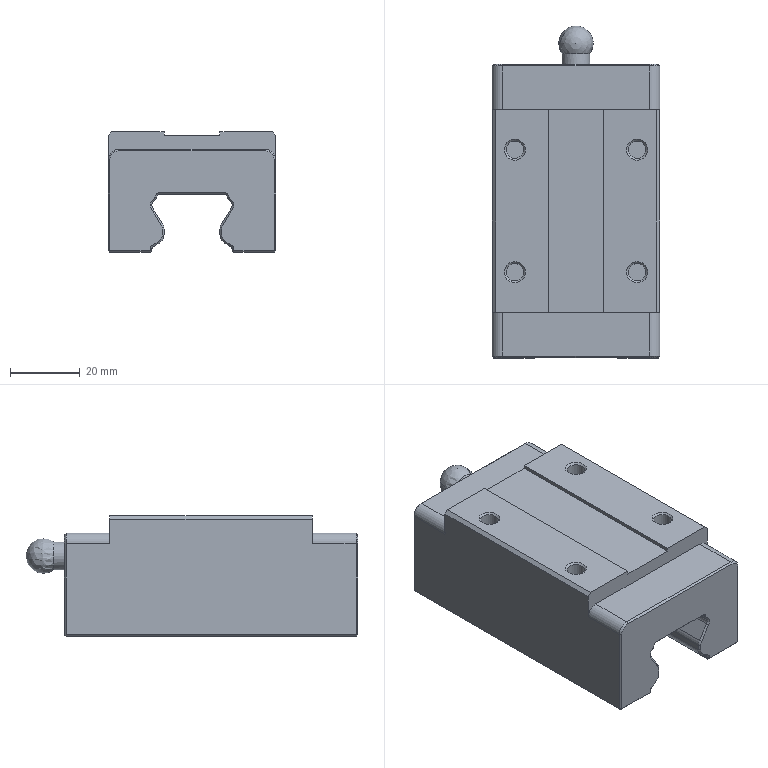Part | STEP file | Tube feed_id1006_x_t | 1 solid | 130 faces | box 48 x 95 x 34.5 mm | volume 104775 mm3 | plane 70 | cone 36 | cylinder 23 | sphere 1 | commonest cylinder face diameters 6 x8 1 x4 3 x4 5 x4 2 x2 8 x1